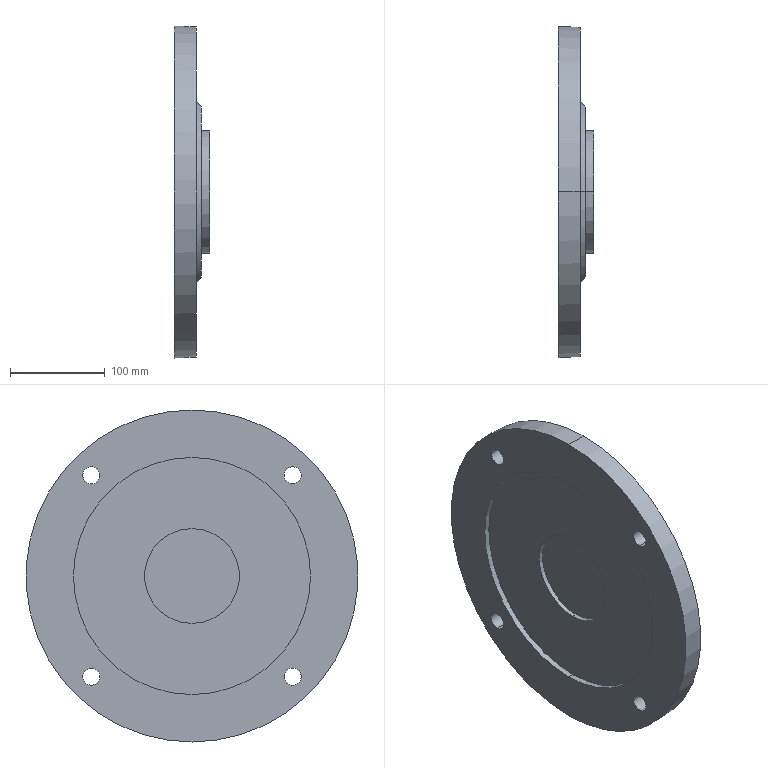Part | STEP file | Input 94 | 1 solid | 24 faces | box 37 x 350 x 350 mm | volume 2104488 mm3 | cylinder 14 | plane 6 | cone 4 | commonest cylinder face diameters 18 x8 100 x2 130 x2 250 x2